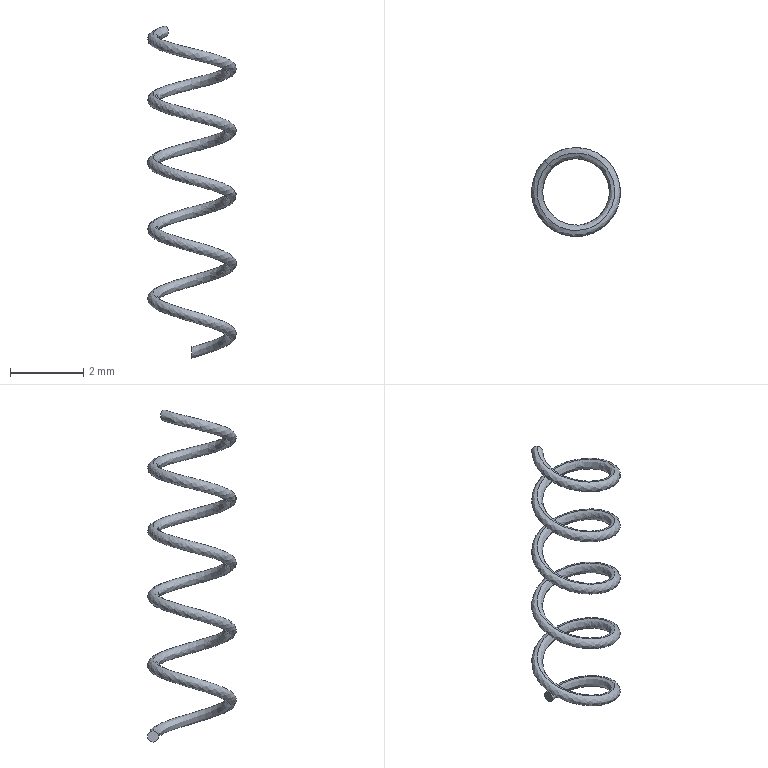Part | SolidWorks | features Helix 1, Sweep 1 | 1 solid | 4 faces | box 2.421 x 2.42 x 9.051 mm | volume 2.291 mm3 | spline 2 | plane 2